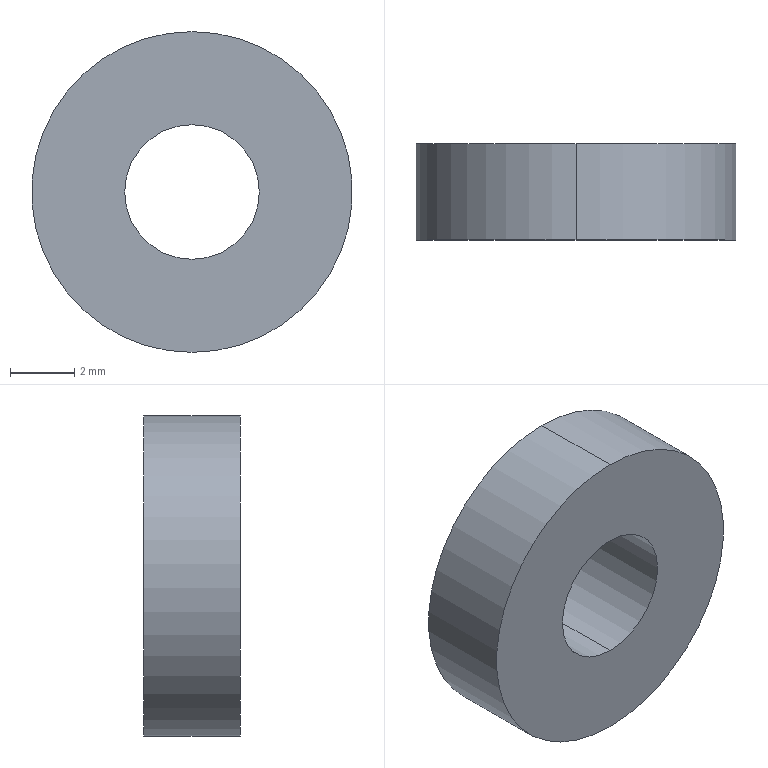Part | SolidWorks | features Extrusion 1 | 1 solid | 6 faces | box 10 x 3 x 10 mm | volume 194.056 mm3 | cylinder 4 | plane 2 | commonest cylinder face diameters 4.2 x2 10 x2
STEP:
#1=CARTESIAN_POINT('',(0.,3.,-2.1));
#2=VERTEX_POINT('',#1);
#3=CARTESIAN_POINT('',(0.,3.,2.1));
#4=VERTEX_POINT('',#3);
#5=CARTESIAN_POINT('',(0.,3.,0.));
#6=DIRECTION('',(0.,1.,0.));
#7=DIRECTION('',(0.,0.,1.));
#8=AXIS2_PLACEMENT_3D('',#5,#6,#7);
#9=CIRCLE('',#8,2.1);
#10=EDGE_CURVE('',#2,#4,#9,.T.);
#11=ORIENTED_EDGE('',*,*,#10,.T.);
#12=CARTESIAN_POINT('',(0.,0.,2.1));
#13=VERTEX_POINT('',#12);
#14=CARTESIAN_POINT('',(0.,3.,2.1));
#15=DIRECTION('',(0.,-1.,0.));
#16=VECTOR('',#15,1000.);
#17=LINE('',#14,#16);
#18=EDGE_CURVE('',#4,#13,#17,.T.);
#19=ORIENTED_EDGE('',*,*,#18,.T.);
#20=CARTESIAN_POINT('',(0.,0.,-2.1));
#21=VERTEX_POINT('',#20);
#22=CARTESIAN_POINT('',(0.,0.,0.));
#23=DIRECTION('',(0.,1.,0.));
#24=DIRECTION('',(0.,0.,1.));
#25=AXIS2_PLACEMENT_3D('',#22,#23,#24);
#26=CIRCLE('',#25,2.1);
#27=EDGE_CURVE('',#21,#13,#26,.T.);
#28=ORIENTED_EDGE('',*,*,#27,.F.);
#29=CARTESIAN_POINT('',(0.,3.,-2.1));
#30=DIRECTION('',(0.,-1.,0.));
#31=VECTOR('',#30,1000.);
#32=LINE('',#29,#31);
#33=EDGE_CURVE('',#2,#21,#32,.T.);
#34=ORIENTED_EDGE('',*,*,#33,.F.);
#35=EDGE_LOOP('',(#11,#19,#28,#34));
#36=FACE_OUTER_BOUND('',#35,.T.);
#37=CARTESIAN_POINT('',(0.,3.,0.));
#38=DIRECTION('',(0.,-1.,0.));
#39=DIRECTION('',(0.,0.,-1.));
#40=AXIS2_PLACEMENT_3D('',#37,#38,#39);
#41=CYLINDRICAL_SURFACE('',#40,2.1);
#42=ADVANCED_FACE('',(#36),#41,.F.);
#43=CARTESIAN_POINT('',(0.,3.,5.));
#44=VERTEX_POINT('',#43);
#45=CARTESIAN_POINT('',(0.,3.,-5.));
#46=VERTEX_POINT('',#45);
#47=CARTESIAN_POINT('',(0.,3.,0.));
#48=DIRECTION('',(0.,1.,0.));
#49=DIRECTION('',(0.,0.,1.));
#50=AXIS2_PLACEMENT_3D('',#47,#48,#49);
#51=CIRCLE('',#50,5.);
#52=EDGE_CURVE('',#44,#46,#51,.T.);
#53=ORIENTED_EDGE('',*,*,#52,.F.);
#54=CARTESIAN_POINT('',(0.,0.,5.));
#55=VERTEX_POINT('',#54);
#56=CARTESIAN_POINT('',(0.,3.,5.));
#57=DIRECTION('',(0.,-1.,0.));
#58=VECTOR('',#57,1000.);
#59=LINE('',#56,#58);
#60=EDGE_CURVE('',#44,#55,#59,.T.);
#61=ORIENTED_EDGE('',*,*,#60,.T.);
#62=CARTESIAN_POINT('',(0.,0.,-5.));
#63=VERTEX_POINT('',#62);
#64=CARTESIAN_POINT('',(0.,0.,0.));
#65=DIRECTION('',(0.,1.,0.));
#66=DIRECTION('',(0.,0.,1.));
#67=AXIS2_PLACEMENT_3D('',#64,#65,#66);
#68=CIRCLE('',#67,5.);
#69=EDGE_CURVE('',#55,#63,#68,.T.);
#70=ORIENTED_EDGE('',*,*,#69,.T.);
#71=CARTESIAN_POINT('',(0.,3.,-5.));
#72=DIRECTION('',(0.,-1.,0.));
#73=VECTOR('',#72,1000.);
#74=LINE('',#71,#73);
#75=EDGE_CURVE('',#46,#63,#74,.T.);
#76=ORIENTED_EDGE('',*,*,#75,.F.);
#77=EDGE_LOOP('',(#53,#61,#70,#76));
#78=FACE_OUTER_BOUND('',#77,.T.);
#79=CARTESIAN_POINT('',(0.,3.,0.));
#80=DIRECTION('',(0.,-1.,0.));
#81=DIRECTION('',(0.,0.,-1.));
#82=AXIS2_PLACEMENT_3D('',#79,#80,#81);
#83=CYLINDRICAL_SURFACE('',#82,5.);
#84=ADVANCED_FACE('',(#78),#83,.T.);
#85=CARTESIAN_POINT('',(0.,3.,0.));
#86=DIRECTION('',(0.,1.,0.));
#87=DIRECTION('',(0.,0.,1.));
#88=AXIS2_PLACEMENT_3D('',#85,#86,#87);
#89=CIRCLE('',#88,5.);
#90=EDGE_CURVE('',#46,#44,#89,.T.);
#91=ORIENTED_EDGE('',*,*,#90,.T.);
#92=ORIENTED_EDGE('',*,*,#52,.T.);
#93=EDGE_LOOP('',(#91,#92));
#94=FACE_OUTER_BOUND('',#93,.T.);
#95=ORIENTED_EDGE('',*,*,#10,.F.);
#96=CARTESIAN_POINT('',(0.,3.,0.));
#97=DIRECTION('',(0.,1.,0.));
#98=DIRECTION('',(0.,0.,1.));
#99=AXIS2_PLACEMENT_3D('',#96,#97,#98);
#100=CIRCLE('',#99,2.1);
#101=EDGE_CURVE('',#4,#2,#100,.T.);
#102=ORIENTED_EDGE('',*,*,#101,.F.);
#103=EDGE_LOOP('',(#95,#102));
#104=FACE_BOUND('',#103,.T.);
#105=CARTESIAN_POINT('',(0.,3.,0.));
#106=DIRECTION('',(0.,1.,0.));
#107=DIRECTION('',(0.,0.,1.));
#108=AXIS2_PLACEMENT_3D('',#105,#106,#107);
#109=PLANE('',#108);
#110=ADVANCED_FACE('',(#94,#104),#109,.T.);
#111=CARTESIAN_POINT('',(0.,0.,0.));
#112=DIRECTION('',(0.,1.,0.));
#113=DIRECTION('',(0.,0.,1.));
#114=AXIS2_PLACEMENT_3D('',#111,#112,#113);
#115=CIRCLE('',#114,5.);
#116=EDGE_CURVE('',#63,#55,#115,.T.);
#117=ORIENTED_EDGE('',*,*,#116,.F.);
#118=ORIENTED_EDGE('',*,*,#69,.F.);
#119=EDGE_LOOP('',(#117,#118));
#120=FACE_OUTER_BOUND('',#119,.T.);
#121=ORIENTED_EDGE('',*,*,#27,.T.);
#122=CARTESIAN_POINT('',(0.,0.,0.));
#123=DIRECTION('',(0.,1.,0.));
#124=DIRECTION('',(0.,0.,1.));
#125=AXIS2_PLACEMENT_3D('',#122,#123,#124);
#126=CIRCLE('',#125,2.1);
#127=EDGE_CURVE('',#13,#21,#126,.T.);
#128=ORIENTED_EDGE('',*,*,#127,.T.);
#129=EDGE_LOOP('',(#121,#128));
#130=FACE_BOUND('',#129,.T.);
#131=CARTESIAN_POINT('',(0.,0.,0.));
#132=DIRECTION('',(0.,1.,0.));
#133=DIRECTION('',(0.,0.,1.));
#134=AXIS2_PLACEMENT_3D('',#131,#132,#133);
#135=PLANE('',#134);
#136=ADVANCED_FACE('',(#120,#130),#135,.F.);
#137=ORIENTED_EDGE('',*,*,#60,.F.);
#138=ORIENTED_EDGE('',*,*,#90,.F.);
#139=ORIENTED_EDGE('',*,*,#75,.T.);
#140=ORIENTED_EDGE('',*,*,#116,.T.);
#141=EDGE_LOOP('',(#137,#138,#139,#140));
#142=FACE_OUTER_BOUND('',#141,.T.);
#143=CARTESIAN_POINT('',(0.,3.,0.));
#144=DIRECTION('',(0.,-1.,0.));
#145=DIRECTION('',(0.,0.,-1.));
#146=AXIS2_PLACEMENT_3D('',#143,#144,#145);
#147=CYLINDRICAL_SURFACE('',#146,5.);
#148=ADVANCED_FACE('',(#142),#147,.T.);
#149=ORIENTED_EDGE('',*,*,#18,.F.);
#150=ORIENTED_EDGE('',*,*,#101,.T.);
#151=ORIENTED_EDGE('',*,*,#33,.T.);
#152=ORIENTED_EDGE('',*,*,#127,.F.);
#153=EDGE_LOOP('',(#149,#150,#151,#152));
#154=FACE_OUTER_BOUND('',#153,.T.);
#155=CARTESIAN_POINT('',(0.,3.,0.));
#156=DIRECTION('',(0.,-1.,0.));
#157=DIRECTION('',(0.,0.,-1.));
#158=AXIS2_PLACEMENT_3D('',#155,#156,#157);
#159=CYLINDRICAL_SURFACE('',#158,2.1);
#160=ADVANCED_FACE('',(#154),#159,.F.);
#161=CLOSED_SHELL('',(#42,#84,#110,#136,#148,#160));
#162=MANIFOLD_SOLID_BREP('',#161);
#163=CARTESIAN_POINT('',(0.,0.,0.));
#164=DIRECTION('',(0.,0.,1.));
#165=DIRECTION('',(1.,0.,0.));
#166=AXIS2_PLACEMENT_3D('',#163,#164,#165);
#167=(LENGTH_UNIT()NAMED_UNIT(*)SI_UNIT(.MILLI.,.METRE.));
#168=UNCERTAINTY_MEASURE_WITH_UNIT(LENGTH_MEASURE(0.00001),#167,'','');
#169=(NAMED_UNIT(*)PLANE_ANGLE_UNIT()SI_UNIT($,.RADIAN.));
#170=(NAMED_UNIT(*)SI_UNIT($,.STERADIAN.)SOLID_ANGLE_UNIT());
#171=(GEOMETRIC_REPRESENTATION_CONTEXT(3)GLOBAL_UNCERTAINTY_ASSIGNED_CONTEXT((#168))GLOBAL_UNIT_ASSIGNED_CONTEXT((#167,#169,#170))REPRESENTATION_CONTEXT('',''));
#172=ADVANCED_BREP_SHAPE_REPRESENTATION('',(#162,#166),#171);